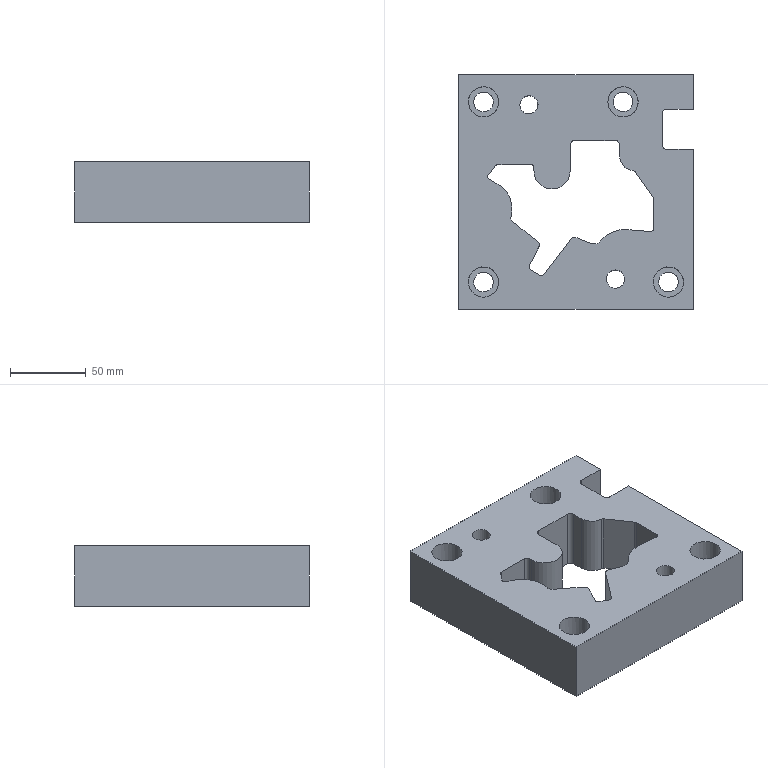Part | STEP file | gslz 2016.10.28-13_id114_x_t | 1 solid | 63 faces | box 155 x 155 x 40 mm | volume 698384 mm3 | plane 32 | cylinder 31 | commonest cylinder face diameters 4 x8 6 x6 20 x5 13 x4 12 x3 40 x2